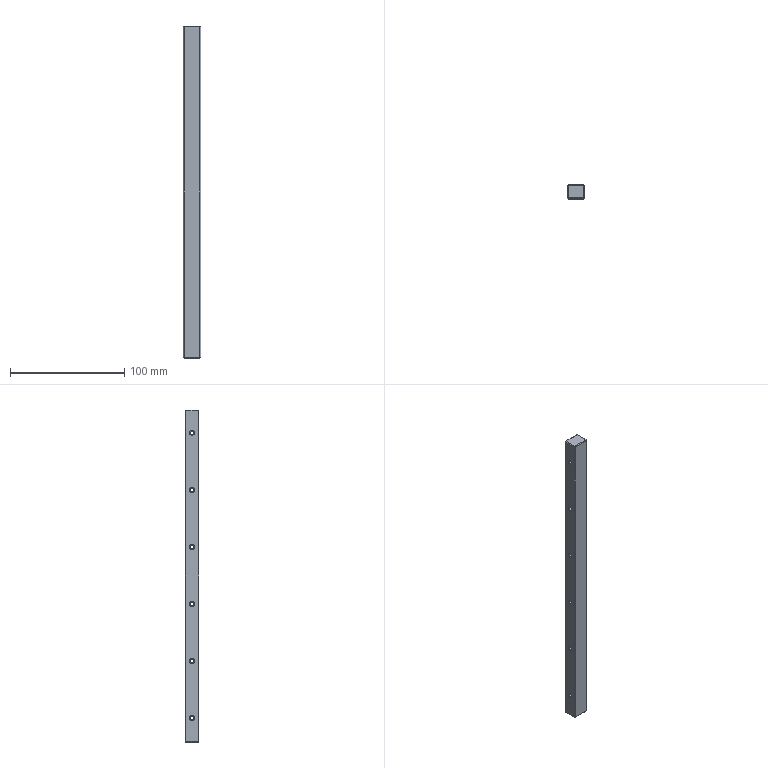Part | STEP file | Circlip fixture-column 2 | 1 solid | 68 faces | box 15 x 12 x 291 mm | volume 51262 mm3 | plane 28 | cone 24 | cylinder 16 | commonest cylinder face diameters 3.3 x16